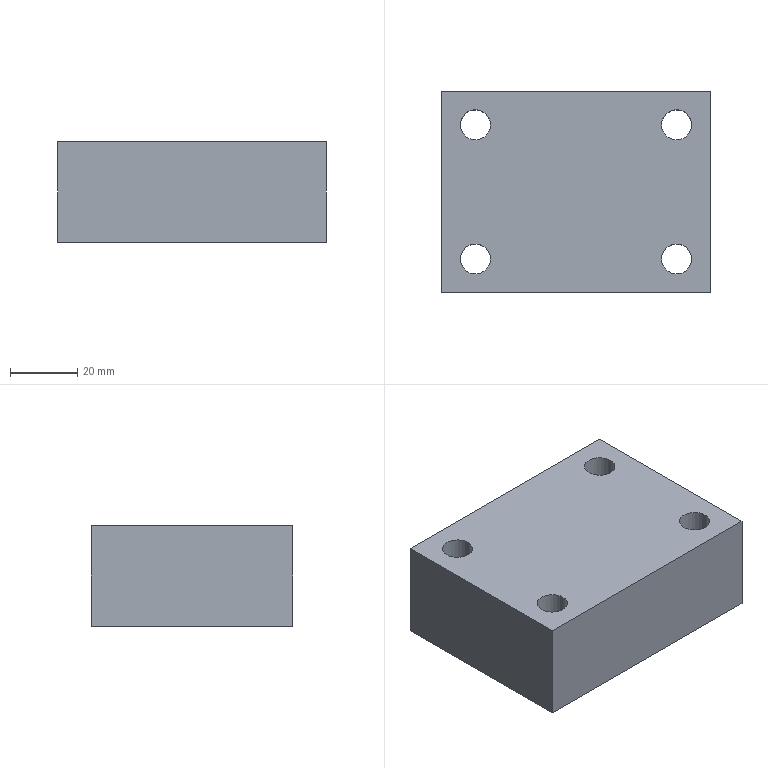Part | SolidWorks | features BaseBody 1 | 1 solid | 14 faces | box 80 x 60 x 30 mm | volume 136366 mm3 | cylinder 8 | plane 6 | commonest cylinder face diameters 9 x8
STEP:
#1=CARTESIAN_POINT('',(-34.5,20.,30.));
#2=VERTEX_POINT('',#1);
#3=CARTESIAN_POINT('',(-25.5,20.,30.));
#4=VERTEX_POINT('',#3);
#5=CARTESIAN_POINT('',(-30.,20.,30.));
#6=DIRECTION('',(0.,0.,1.));
#7=DIRECTION('',(1.,0.,0.));
#8=AXIS2_PLACEMENT_3D('',#5,#6,#7);
#9=CIRCLE('',#8,4.5);
#10=EDGE_CURVE('',#2,#4,#9,.T.);
#11=ORIENTED_EDGE('',*,*,#10,.T.);
#12=CARTESIAN_POINT('',(-25.5,20.,0.));
#13=VERTEX_POINT('',#12);
#14=CARTESIAN_POINT('',(-25.5,20.,30.));
#15=DIRECTION('',(0.,0.,-1.));
#16=VECTOR('',#15,1000.);
#17=LINE('',#14,#16);
#18=EDGE_CURVE('',#4,#13,#17,.T.);
#19=ORIENTED_EDGE('',*,*,#18,.T.);
#20=CARTESIAN_POINT('',(-34.5,20.,0.));
#21=VERTEX_POINT('',#20);
#22=CARTESIAN_POINT('',(-30.,20.,0.));
#23=DIRECTION('',(0.,0.,1.));
#24=DIRECTION('',(1.,0.,0.));
#25=AXIS2_PLACEMENT_3D('',#22,#23,#24);
#26=CIRCLE('',#25,4.5);
#27=EDGE_CURVE('',#21,#13,#26,.T.);
#28=ORIENTED_EDGE('',*,*,#27,.F.);
#29=CARTESIAN_POINT('',(-34.5,20.,30.));
#30=DIRECTION('',(0.,0.,-1.));
#31=VECTOR('',#30,1000.);
#32=LINE('',#29,#31);
#33=EDGE_CURVE('',#2,#21,#32,.T.);
#34=ORIENTED_EDGE('',*,*,#33,.F.);
#35=EDGE_LOOP('',(#11,#19,#28,#34));
#36=FACE_OUTER_BOUND('',#35,.T.);
#37=CARTESIAN_POINT('',(-30.,20.,30.));
#38=DIRECTION('',(0.,0.,-1.));
#39=DIRECTION('',(-1.,0.,0.));
#40=AXIS2_PLACEMENT_3D('',#37,#38,#39);
#41=CYLINDRICAL_SURFACE('',#40,4.5);
#42=ADVANCED_FACE('',(#36),#41,.F.);
#43=CARTESIAN_POINT('',(-34.5,-20.,30.));
#44=VERTEX_POINT('',#43);
#45=CARTESIAN_POINT('',(-25.5,-20.,30.));
#46=VERTEX_POINT('',#45);
#47=CARTESIAN_POINT('',(-30.,-20.,30.));
#48=DIRECTION('',(0.,0.,1.));
#49=DIRECTION('',(1.,0.,0.));
#50=AXIS2_PLACEMENT_3D('',#47,#48,#49);
#51=CIRCLE('',#50,4.5);
#52=EDGE_CURVE('',#44,#46,#51,.T.);
#53=ORIENTED_EDGE('',*,*,#52,.T.);
#54=CARTESIAN_POINT('',(-25.5,-20.,0.));
#55=VERTEX_POINT('',#54);
#56=CARTESIAN_POINT('',(-25.5,-20.,30.));
#57=DIRECTION('',(0.,0.,-1.));
#58=VECTOR('',#57,1000.);
#59=LINE('',#56,#58);
#60=EDGE_CURVE('',#46,#55,#59,.T.);
#61=ORIENTED_EDGE('',*,*,#60,.T.);
#62=CARTESIAN_POINT('',(-34.5,-20.,0.));
#63=VERTEX_POINT('',#62);
#64=CARTESIAN_POINT('',(-30.,-20.,0.));
#65=DIRECTION('',(0.,0.,1.));
#66=DIRECTION('',(1.,0.,0.));
#67=AXIS2_PLACEMENT_3D('',#64,#65,#66);
#68=CIRCLE('',#67,4.5);
#69=EDGE_CURVE('',#63,#55,#68,.T.);
#70=ORIENTED_EDGE('',*,*,#69,.F.);
#71=CARTESIAN_POINT('',(-34.5,-20.,30.));
#72=DIRECTION('',(0.,0.,-1.));
#73=VECTOR('',#72,1000.);
#74=LINE('',#71,#73);
#75=EDGE_CURVE('',#44,#63,#74,.T.);
#76=ORIENTED_EDGE('',*,*,#75,.F.);
#77=EDGE_LOOP('',(#53,#61,#70,#76));
#78=FACE_OUTER_BOUND('',#77,.T.);
#79=CARTESIAN_POINT('',(-30.,-20.,30.));
#80=DIRECTION('',(0.,0.,-1.));
#81=DIRECTION('',(-1.,0.,0.));
#82=AXIS2_PLACEMENT_3D('',#79,#80,#81);
#83=CYLINDRICAL_SURFACE('',#82,4.5);
#84=ADVANCED_FACE('',(#78),#83,.F.);
#85=CARTESIAN_POINT('',(25.5,20.,30.));
#86=VERTEX_POINT('',#85);
#87=CARTESIAN_POINT('',(34.5,20.,30.));
#88=VERTEX_POINT('',#87);
#89=CARTESIAN_POINT('',(30.,20.,30.));
#90=DIRECTION('',(0.,0.,1.));
#91=DIRECTION('',(1.,0.,0.));
#92=AXIS2_PLACEMENT_3D('',#89,#90,#91);
#93=CIRCLE('',#92,4.5);
#94=EDGE_CURVE('',#86,#88,#93,.T.);
#95=ORIENTED_EDGE('',*,*,#94,.T.);
#96=CARTESIAN_POINT('',(34.5,20.,0.));
#97=VERTEX_POINT('',#96);
#98=CARTESIAN_POINT('',(34.5,20.,30.));
#99=DIRECTION('',(0.,0.,-1.));
#100=VECTOR('',#99,1000.);
#101=LINE('',#98,#100);
#102=EDGE_CURVE('',#88,#97,#101,.T.);
#103=ORIENTED_EDGE('',*,*,#102,.T.);
#104=CARTESIAN_POINT('',(25.5,20.,0.));
#105=VERTEX_POINT('',#104);
#106=CARTESIAN_POINT('',(30.,20.,0.));
#107=DIRECTION('',(0.,0.,1.));
#108=DIRECTION('',(1.,0.,0.));
#109=AXIS2_PLACEMENT_3D('',#106,#107,#108);
#110=CIRCLE('',#109,4.5);
#111=EDGE_CURVE('',#105,#97,#110,.T.);
#112=ORIENTED_EDGE('',*,*,#111,.F.);
#113=CARTESIAN_POINT('',(25.5,20.,30.));
#114=DIRECTION('',(0.,0.,-1.));
#115=VECTOR('',#114,1000.);
#116=LINE('',#113,#115);
#117=EDGE_CURVE('',#86,#105,#116,.T.);
#118=ORIENTED_EDGE('',*,*,#117,.F.);
#119=EDGE_LOOP('',(#95,#103,#112,#118));
#120=FACE_OUTER_BOUND('',#119,.T.);
#121=CARTESIAN_POINT('',(30.,20.,30.));
#122=DIRECTION('',(0.,0.,-1.));
#123=DIRECTION('',(-1.,0.,0.));
#124=AXIS2_PLACEMENT_3D('',#121,#122,#123);
#125=CYLINDRICAL_SURFACE('',#124,4.5);
#126=ADVANCED_FACE('',(#120),#125,.F.);
#127=CARTESIAN_POINT('',(25.5,-20.,30.));
#128=VERTEX_POINT('',#127);
#129=CARTESIAN_POINT('',(34.5,-20.,30.));
#130=VERTEX_POINT('',#129);
#131=CARTESIAN_POINT('',(30.,-20.,30.));
#132=DIRECTION('',(0.,0.,1.));
#133=DIRECTION('',(1.,0.,0.));
#134=AXIS2_PLACEMENT_3D('',#131,#132,#133);
#135=CIRCLE('',#134,4.5);
#136=EDGE_CURVE('',#128,#130,#135,.T.);
#137=ORIENTED_EDGE('',*,*,#136,.T.);
#138=CARTESIAN_POINT('',(34.5,-20.,0.));
#139=VERTEX_POINT('',#138);
#140=CARTESIAN_POINT('',(34.5,-20.,30.));
#141=DIRECTION('',(0.,0.,-1.));
#142=VECTOR('',#141,1000.);
#143=LINE('',#140,#142);
#144=EDGE_CURVE('',#130,#139,#143,.T.);
#145=ORIENTED_EDGE('',*,*,#144,.T.);
#146=CARTESIAN_POINT('',(25.5,-20.,0.));
#147=VERTEX_POINT('',#146);
#148=CARTESIAN_POINT('',(30.,-20.,0.));
#149=DIRECTION('',(0.,0.,1.));
#150=DIRECTION('',(1.,0.,0.));
#151=AXIS2_PLACEMENT_3D('',#148,#149,#150);
#152=CIRCLE('',#151,4.5);
#153=EDGE_CURVE('',#147,#139,#152,.T.);
#154=ORIENTED_EDGE('',*,*,#153,.F.);
#155=CARTESIAN_POINT('',(25.5,-20.,30.));
#156=DIRECTION('',(0.,0.,-1.));
#157=VECTOR('',#156,1000.);
#158=LINE('',#155,#157);
#159=EDGE_CURVE('',#128,#147,#158,.T.);
#160=ORIENTED_EDGE('',*,*,#159,.F.);
#161=EDGE_LOOP('',(#137,#145,#154,#160));
#162=FACE_OUTER_BOUND('',#161,.T.);
#163=CARTESIAN_POINT('',(30.,-20.,30.));
#164=DIRECTION('',(0.,0.,-1.));
#165=DIRECTION('',(-1.,0.,0.));
#166=AXIS2_PLACEMENT_3D('',#163,#164,#165);
#167=CYLINDRICAL_SURFACE('',#166,4.5);
#168=ADVANCED_FACE('',(#162),#167,.F.);
#169=CARTESIAN_POINT('',(-40.,-30.,0.));
#170=VERTEX_POINT('',#169);
#171=CARTESIAN_POINT('',(-40.,30.,0.));
#172=VERTEX_POINT('',#171);
#173=CARTESIAN_POINT('',(-40.,0.,0.));
#174=DIRECTION('',(0.,1.,0.));
#175=VECTOR('',#174,1000.);
#176=LINE('',#173,#175);
#177=EDGE_CURVE('',#170,#172,#176,.T.);
#178=ORIENTED_EDGE('',*,*,#177,.F.);
#179=CARTESIAN_POINT('',(-40.,-30.,30.));
#180=VERTEX_POINT('',#179);
#181=CARTESIAN_POINT('',(-40.,-30.,30.));
#182=DIRECTION('',(0.,0.,-1.));
#183=VECTOR('',#182,1000.);
#184=LINE('',#181,#183);
#185=EDGE_CURVE('',#180,#170,#184,.T.);
#186=ORIENTED_EDGE('',*,*,#185,.F.);
#187=CARTESIAN_POINT('',(-40.,30.,30.));
#188=VERTEX_POINT('',#187);
#189=CARTESIAN_POINT('',(-40.,0.,30.));
#190=DIRECTION('',(0.,1.,0.));
#191=VECTOR('',#190,1000.);
#192=LINE('',#189,#191);
#193=EDGE_CURVE('',#180,#188,#192,.T.);
#194=ORIENTED_EDGE('',*,*,#193,.T.);
#195=CARTESIAN_POINT('',(-40.,30.,30.));
#196=DIRECTION('',(0.,0.,-1.));
#197=VECTOR('',#196,1000.);
#198=LINE('',#195,#197);
#199=EDGE_CURVE('',#188,#172,#198,.T.);
#200=ORIENTED_EDGE('',*,*,#199,.T.);
#201=EDGE_LOOP('',(#178,#186,#194,#200));
#202=FACE_OUTER_BOUND('',#201,.T.);
#203=CARTESIAN_POINT('',(-40.,0.,30.));
#204=DIRECTION('',(-1.,0.,0.));
#205=DIRECTION('',(0.,0.,1.));
#206=AXIS2_PLACEMENT_3D('',#203,#204,#205);
#207=PLANE('',#206);
#208=ADVANCED_FACE('',(#202),#207,.T.);
#209=CARTESIAN_POINT('',(40.,-30.,0.));
#210=VERTEX_POINT('',#209);
#211=CARTESIAN_POINT('',(0.,-30.,0.));
#212=DIRECTION('',(-1.,0.,0.));
#213=VECTOR('',#212,1000.);
#214=LINE('',#211,#213);
#215=EDGE_CURVE('',#210,#170,#214,.T.);
#216=ORIENTED_EDGE('',*,*,#215,.F.);
#217=CARTESIAN_POINT('',(40.,-30.,30.));
#218=VERTEX_POINT('',#217);
#219=CARTESIAN_POINT('',(40.,-30.,30.));
#220=DIRECTION('',(0.,0.,-1.));
#221=VECTOR('',#220,1000.);
#222=LINE('',#219,#221);
#223=EDGE_CURVE('',#218,#210,#222,.T.);
#224=ORIENTED_EDGE('',*,*,#223,.F.);
#225=CARTESIAN_POINT('',(0.,-30.,30.));
#226=DIRECTION('',(-1.,0.,0.));
#227=VECTOR('',#226,1000.);
#228=LINE('',#225,#227);
#229=EDGE_CURVE('',#218,#180,#228,.T.);
#230=ORIENTED_EDGE('',*,*,#229,.T.);
#231=ORIENTED_EDGE('',*,*,#185,.T.);
#232=EDGE_LOOP('',(#216,#224,#230,#231));
#233=FACE_OUTER_BOUND('',#232,.T.);
#234=CARTESIAN_POINT('',(0.,-30.,30.));
#235=DIRECTION('',(0.,-1.,0.));
#236=DIRECTION('',(1.,0.,0.));
#237=AXIS2_PLACEMENT_3D('',#234,#235,#236);
#238=PLANE('',#237);
#239=ADVANCED_FACE('',(#233),#238,.T.);
#240=CARTESIAN_POINT('',(40.,30.,0.));
#241=VERTEX_POINT('',#240);
#242=CARTESIAN_POINT('',(40.,0.,0.));
#243=DIRECTION('',(0.,1.,0.));
#244=VECTOR('',#243,1000.);
#245=LINE('',#242,#244);
#246=EDGE_CURVE('',#210,#241,#245,.T.);
#247=ORIENTED_EDGE('',*,*,#246,.T.);
#248=CARTESIAN_POINT('',(40.,30.,30.));
#249=VERTEX_POINT('',#248);
#250=CARTESIAN_POINT('',(40.,30.,30.));
#251=DIRECTION('',(0.,0.,-1.));
#252=VECTOR('',#251,1000.);
#253=LINE('',#250,#252);
#254=EDGE_CURVE('',#249,#241,#253,.T.);
#255=ORIENTED_EDGE('',*,*,#254,.F.);
#256=CARTESIAN_POINT('',(40.,0.,30.));
#257=DIRECTION('',(0.,1.,0.));
#258=VECTOR('',#257,1000.);
#259=LINE('',#256,#258);
#260=EDGE_CURVE('',#218,#249,#259,.T.);
#261=ORIENTED_EDGE('',*,*,#260,.F.);
#262=ORIENTED_EDGE('',*,*,#223,.T.);
#263=EDGE_LOOP('',(#247,#255,#261,#262));
#264=FACE_OUTER_BOUND('',#263,.T.);
#265=CARTESIAN_POINT('',(40.,0.,30.));
#266=DIRECTION('',(-1.,0.,0.));
#267=DIRECTION('',(0.,0.,1.));
#268=AXIS2_PLACEMENT_3D('',#265,#266,#267);
#269=PLANE('',#268);
#270=ADVANCED_FACE('',(#264),#269,.F.);
#271=ORIENTED_EDGE('',*,*,#144,.F.);
#272=CARTESIAN_POINT('',(30.,-20.,30.));
#273=DIRECTION('',(0.,0.,1.));
#274=DIRECTION('',(1.,0.,0.));
#275=AXIS2_PLACEMENT_3D('',#272,#273,#274);
#276=CIRCLE('',#275,4.5);
#277=EDGE_CURVE('',#130,#128,#276,.T.);
#278=ORIENTED_EDGE('',*,*,#277,.T.);
#279=ORIENTED_EDGE('',*,*,#159,.T.);
#280=CARTESIAN_POINT('',(30.,-20.,0.));
#281=DIRECTION('',(0.,0.,1.));
#282=DIRECTION('',(1.,0.,0.));
#283=AXIS2_PLACEMENT_3D('',#280,#281,#282);
#284=CIRCLE('',#283,4.5);
#285=EDGE_CURVE('',#139,#147,#284,.T.);
#286=ORIENTED_EDGE('',*,*,#285,.F.);
#287=EDGE_LOOP('',(#271,#278,#279,#286));
#288=FACE_OUTER_BOUND('',#287,.T.);
#289=CARTESIAN_POINT('',(30.,-20.,30.));
#290=DIRECTION('',(0.,0.,-1.));
#291=DIRECTION('',(-1.,0.,0.));
#292=AXIS2_PLACEMENT_3D('',#289,#290,#291);
#293=CYLINDRICAL_SURFACE('',#292,4.5);
#294=ADVANCED_FACE('',(#288),#293,.F.);
#295=ORIENTED_EDGE('',*,*,#102,.F.);
#296=CARTESIAN_POINT('',(30.,20.,30.));
#297=DIRECTION('',(0.,0.,1.));
#298=DIRECTION('',(1.,0.,0.));
#299=AXIS2_PLACEMENT_3D('',#296,#297,#298);
#300=CIRCLE('',#299,4.5);
#301=EDGE_CURVE('',#88,#86,#300,.T.);
#302=ORIENTED_EDGE('',*,*,#301,.T.);
#303=ORIENTED_EDGE('',*,*,#117,.T.);
#304=CARTESIAN_POINT('',(30.,20.,0.));
#305=DIRECTION('',(0.,0.,1.));
#306=DIRECTION('',(1.,0.,0.));
#307=AXIS2_PLACEMENT_3D('',#304,#305,#306);
#308=CIRCLE('',#307,4.5);
#309=EDGE_CURVE('',#97,#105,#308,.T.);
#310=ORIENTED_EDGE('',*,*,#309,.F.);
#311=EDGE_LOOP('',(#295,#302,#303,#310));
#312=FACE_OUTER_BOUND('',#311,.T.);
#313=CARTESIAN_POINT('',(30.,20.,30.));
#314=DIRECTION('',(0.,0.,-1.));
#315=DIRECTION('',(-1.,0.,0.));
#316=AXIS2_PLACEMENT_3D('',#313,#314,#315);
#317=CYLINDRICAL_SURFACE('',#316,4.5);
#318=ADVANCED_FACE('',(#312),#317,.F.);
#319=ORIENTED_EDGE('',*,*,#60,.F.);
#320=CARTESIAN_POINT('',(-30.,-20.,30.));
#321=DIRECTION('',(0.,0.,1.));
#322=DIRECTION('',(1.,0.,0.));
#323=AXIS2_PLACEMENT_3D('',#320,#321,#322);
#324=CIRCLE('',#323,4.5);
#325=EDGE_CURVE('',#46,#44,#324,.T.);
#326=ORIENTED_EDGE('',*,*,#325,.T.);
#327=ORIENTED_EDGE('',*,*,#75,.T.);
#328=CARTESIAN_POINT('',(-30.,-20.,0.));
#329=DIRECTION('',(0.,0.,1.));
#330=DIRECTION('',(1.,0.,0.));
#331=AXIS2_PLACEMENT_3D('',#328,#329,#330);
#332=CIRCLE('',#331,4.5);
#333=EDGE_CURVE('',#55,#63,#332,.T.);
#334=ORIENTED_EDGE('',*,*,#333,.F.);
#335=EDGE_LOOP('',(#319,#326,#327,#334));
#336=FACE_OUTER_BOUND('',#335,.T.);
#337=CARTESIAN_POINT('',(-30.,-20.,30.));
#338=DIRECTION('',(0.,0.,-1.));
#339=DIRECTION('',(-1.,0.,0.));
#340=AXIS2_PLACEMENT_3D('',#337,#338,#339);
#341=CYLINDRICAL_SURFACE('',#340,4.5);
#342=ADVANCED_FACE('',(#336),#341,.F.);
#343=ORIENTED_EDGE('',*,*,#18,.F.);
#344=CARTESIAN_POINT('',(-30.,20.,30.));
#345=DIRECTION('',(0.,0.,1.));
#346=DIRECTION('',(1.,0.,0.));
#347=AXIS2_PLACEMENT_3D('',#344,#345,#346);
#348=CIRCLE('',#347,4.5);
#349=EDGE_CURVE('',#4,#2,#348,.T.);
#350=ORIENTED_EDGE('',*,*,#349,.T.);
#351=ORIENTED_EDGE('',*,*,#33,.T.);
#352=CARTESIAN_POINT('',(-30.,20.,0.));
#353=DIRECTION('',(0.,0.,1.));
#354=DIRECTION('',(1.,0.,0.));
#355=AXIS2_PLACEMENT_3D('',#352,#353,#354);
#356=CIRCLE('',#355,4.5);
#357=EDGE_CURVE('',#13,#21,#356,.T.);
#358=ORIENTED_EDGE('',*,*,#357,.F.);
#359=EDGE_LOOP('',(#343,#350,#351,#358));
#360=FACE_OUTER_BOUND('',#359,.T.);
#361=CARTESIAN_POINT('',(-30.,20.,30.));
#362=DIRECTION('',(0.,0.,-1.));
#363=DIRECTION('',(-1.,0.,0.));
#364=AXIS2_PLACEMENT_3D('',#361,#362,#363);
#365=CYLINDRICAL_SURFACE('',#364,4.5);
#366=ADVANCED_FACE('',(#360),#365,.F.);
#367=CARTESIAN_POINT('',(0.,30.,0.));
#368=DIRECTION('',(-1.,0.,0.));
#369=VECTOR('',#368,1000.);
#370=LINE('',#367,#369);
#371=EDGE_CURVE('',#241,#172,#370,.T.);
#372=ORIENTED_EDGE('',*,*,#371,.T.);
#373=ORIENTED_EDGE('',*,*,#199,.F.);
#374=CARTESIAN_POINT('',(0.,30.,30.));
#375=DIRECTION('',(-1.,0.,0.));
#376=VECTOR('',#375,1000.);
#377=LINE('',#374,#376);
#378=EDGE_CURVE('',#249,#188,#377,.T.);
#379=ORIENTED_EDGE('',*,*,#378,.F.);
#380=ORIENTED_EDGE('',*,*,#254,.T.);
#381=EDGE_LOOP('',(#372,#373,#379,#380));
#382=FACE_OUTER_BOUND('',#381,.T.);
#383=CARTESIAN_POINT('',(0.,30.,30.));
#384=DIRECTION('',(0.,-1.,0.));
#385=DIRECTION('',(1.,0.,0.));
#386=AXIS2_PLACEMENT_3D('',#383,#384,#385);
#387=PLANE('',#386);
#388=ADVANCED_FACE('',(#382),#387,.F.);
#389=ORIENTED_EDGE('',*,*,#10,.F.);
#390=ORIENTED_EDGE('',*,*,#349,.F.);
#391=EDGE_LOOP('',(#389,#390));
#392=FACE_BOUND('',#391,.T.);
#393=ORIENTED_EDGE('',*,*,#52,.F.);
#394=ORIENTED_EDGE('',*,*,#325,.F.);
#395=EDGE_LOOP('',(#393,#394));
#396=FACE_BOUND('',#395,.T.);
#397=ORIENTED_EDGE('',*,*,#94,.F.);
#398=ORIENTED_EDGE('',*,*,#301,.F.);
#399=EDGE_LOOP('',(#397,#398));
#400=FACE_BOUND('',#399,.T.);
#401=ORIENTED_EDGE('',*,*,#136,.F.);
#402=ORIENTED_EDGE('',*,*,#277,.F.);
#403=EDGE_LOOP('',(#401,#402));
#404=FACE_BOUND('',#403,.T.);
#405=ORIENTED_EDGE('',*,*,#193,.F.);
#406=ORIENTED_EDGE('',*,*,#229,.F.);
#407=ORIENTED_EDGE('',*,*,#260,.T.);
#408=ORIENTED_EDGE('',*,*,#378,.T.);
#409=EDGE_LOOP('',(#405,#406,#407,#408));
#410=FACE_OUTER_BOUND('',#409,.T.);
#411=CARTESIAN_POINT('',(0.,0.,30.));
#412=DIRECTION('',(0.,0.,1.));
#413=DIRECTION('',(1.,0.,0.));
#414=AXIS2_PLACEMENT_3D('',#411,#412,#413);
#415=PLANE('',#414);
#416=ADVANCED_FACE('',(#392,#396,#400,#404,#410),#415,.T.);
#417=ORIENTED_EDGE('',*,*,#27,.T.);
#418=ORIENTED_EDGE('',*,*,#357,.T.);
#419=EDGE_LOOP('',(#417,#418));
#420=FACE_BOUND('',#419,.T.);
#421=ORIENTED_EDGE('',*,*,#69,.T.);
#422=ORIENTED_EDGE('',*,*,#333,.T.);
#423=EDGE_LOOP('',(#421,#422));
#424=FACE_BOUND('',#423,.T.);
#425=ORIENTED_EDGE('',*,*,#111,.T.);
#426=ORIENTED_EDGE('',*,*,#309,.T.);
#427=EDGE_LOOP('',(#425,#426));
#428=FACE_BOUND('',#427,.T.);
#429=ORIENTED_EDGE('',*,*,#153,.T.);
#430=ORIENTED_EDGE('',*,*,#285,.T.);
#431=EDGE_LOOP('',(#429,#430));
#432=FACE_BOUND('',#431,.T.);
#433=ORIENTED_EDGE('',*,*,#177,.T.);
#434=ORIENTED_EDGE('',*,*,#371,.F.);
#435=ORIENTED_EDGE('',*,*,#246,.F.);
#436=ORIENTED_EDGE('',*,*,#215,.T.);
#437=EDGE_LOOP('',(#433,#434,#435,#436));
#438=FACE_OUTER_BOUND('',#437,.T.);
#439=CARTESIAN_POINT('',(0.,0.,0.));
#440=DIRECTION('',(0.,0.,1.));
#441=DIRECTION('',(1.,0.,0.));
#442=AXIS2_PLACEMENT_3D('',#439,#440,#441);
#443=PLANE('',#442);
#444=ADVANCED_FACE('',(#420,#424,#428,#432,#438),#443,.F.);
#445=CLOSED_SHELL('',(#42,#84,#126,#168,#208,#239,#270,#294,#318,#342,#366,#388,#416,#444));
#446=MANIFOLD_SOLID_BREP('',#445);
#447=CARTESIAN_POINT('',(0.,0.,0.));
#448=DIRECTION('',(0.,0.,1.));
#449=DIRECTION('',(1.,0.,0.));
#450=AXIS2_PLACEMENT_3D('',#447,#448,#449);
#451=(LENGTH_UNIT()NAMED_UNIT(*)SI_UNIT(.MILLI.,.METRE.));
#452=UNCERTAINTY_MEASURE_WITH_UNIT(LENGTH_MEASURE(0.00001),#451,'','');
#453=(NAMED_UNIT(*)PLANE_ANGLE_UNIT()SI_UNIT($,.RADIAN.));
#454=(NAMED_UNIT(*)SI_UNIT($,.STERADIAN.)SOLID_ANGLE_UNIT());
#455=(GEOMETRIC_REPRESENTATION_CONTEXT(3)GLOBAL_UNCERTAINTY_ASSIGNED_CONTEXT((#452))GLOBAL_UNIT_ASSIGNED_CONTEXT((#451,#453,#454))REPRESENTATION_CONTEXT('',''));
#456=ADVANCED_BREP_SHAPE_REPRESENTATION('',(#446,#450),#455);